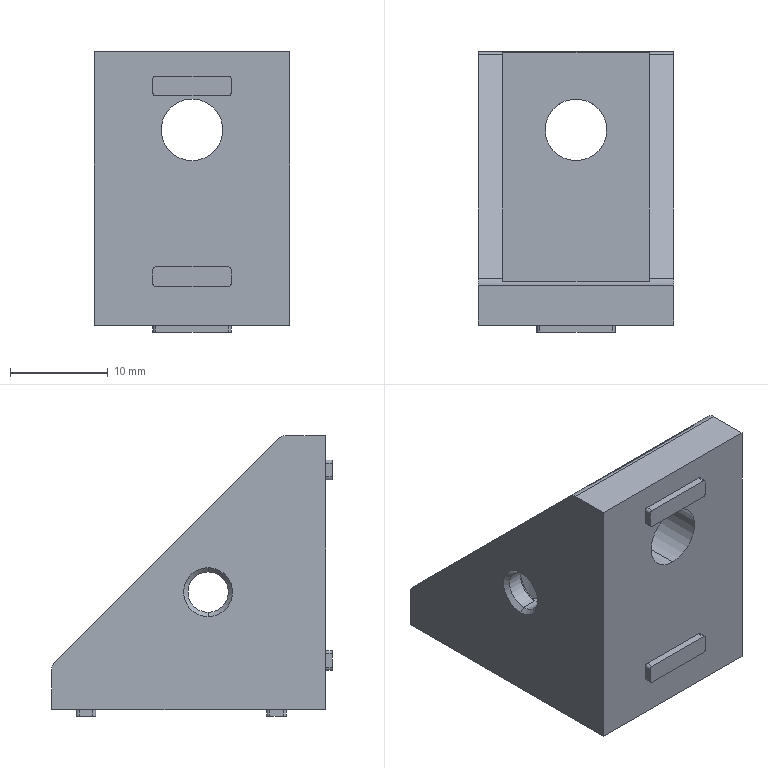Part | STEP file | 1 solid | 66 faces | box 20 x 28.7 x 28.7 mm | volume 5707 mm3 | plane 32 | cylinder 26 | cone 8 | commonest cylinder face diameters 0.6 x16 4.134 x4 6.3 x4 2 x2